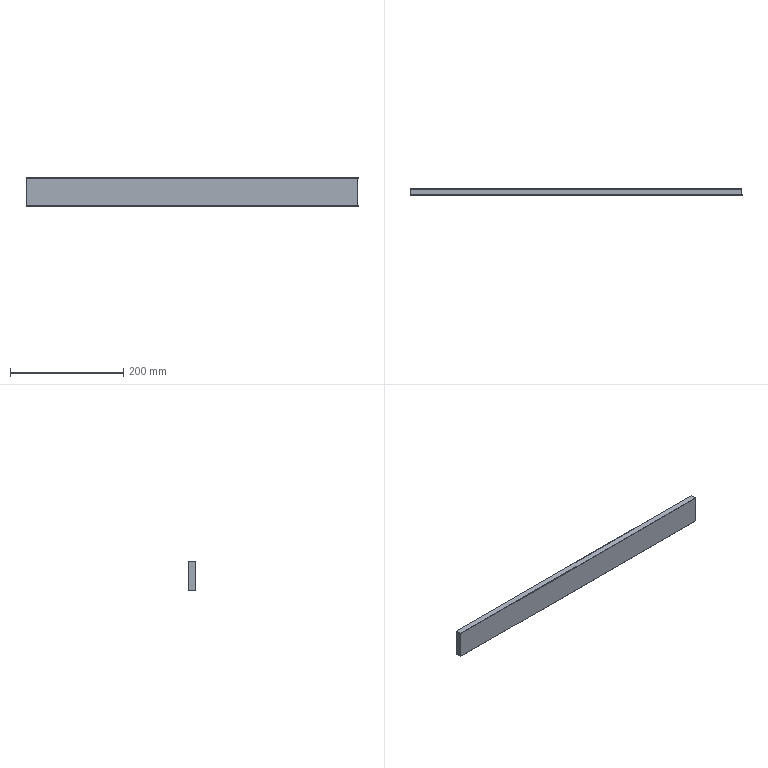Part | STEP file | DEWALT-DWE7492-B22 | 1 solid | 10 faces | box 586.2 x 11 x 50 mm | volume 322284 mm3 | plane 6 | cylinder 4 | commonest cylinder face diameters 1 x4
STEP:
#1=CARTESIAN_POINT('',(0.,0.,0.));
#2=DIRECTION('',(0.,0.,1.));
#3=DIRECTION('',(1.,0.,0.));
#4=AXIS2_PLACEMENT_3D('',#1,#2,#3);
#5=CARTESIAN_POINT('',(-302.1,210.8,45.5));
#6=VERTEX_POINT('',#5);
#7=CARTESIAN_POINT('',(-302.1,211.3,45.));
#8=VERTEX_POINT('',#7);
#9=CARTESIAN_POINT('',(-302.1,211.3,45.5));
#10=DIRECTION('',(1.,0.,0.));
#11=DIRECTION('',(0.,-1.,0.));
#12=AXIS2_PLACEMENT_3D('',#9,#10,#11);
#13=CIRCLE('',#12,0.5);
#14=CARTESIAN_POINT('',(-302.1,211.3,45.5));
#15=DIRECTION('',(1.,0.,0.));
#16=DIRECTION('',(0.,0.,-1.));
#17=AXIS2_PLACEMENT_3D('',#14,#15,#16);
#18=CYLINDRICAL_SURFACE('',#17,0.5);
#19=CARTESIAN_POINT('',(4.712,0.));
#20=DIRECTION('',(1.,0.));
#21=VECTOR('',#20,1.);
#22=LINE('',#19,#21);
#23=(GEOMETRIC_REPRESENTATION_CONTEXT(2)PARAMETRIC_REPRESENTATION_CONTEXT()REPRESENTATION_CONTEXT('',''));
#24=DEFINITIONAL_REPRESENTATION('',(#22),#23);
#25=PCURVE('',#18,#24);
#26=CARTESIAN_POINT('',(-302.1,210.79,44.99));
#27=DIRECTION('',(-1.,0.,0.));
#28=DIRECTION('',(0.,0.,1.));
#29=AXIS2_PLACEMENT_3D('',#26,#27,#28);
#30=PLANE('',#29);
#31=CARTESIAN_POINT('',(0.51,0.01));
#32=CARTESIAN_POINT('',(-0.356,0.01));
#33=CARTESIAN_POINT('',(0.07699,0.76));
#34=CARTESIAN_POINT('',(0.51,1.51));
#35=CARTESIAN_POINT('',(0.943,0.76));
#36=CARTESIAN_POINT('',(1.376,0.01));
#37=CARTESIAN_POINT('',(0.51,0.01));
#38=(BOUNDED_CURVE()B_SPLINE_CURVE(2,(#31,#32,#33,#34,#35,#36,#37),.UNSPECIFIED.,.T.,.F.)B_SPLINE_CURVE_WITH_KNOTS((1,2,2,2,2,1),(-2.094,0.,2.094,4.189,6.283,8.378),.UNSPECIFIED.)CURVE()GEOMETRIC_REPRESENTATION_ITEM()RATIONAL_B_SPLINE_CURVE((1.,0.5,1.,0.5,1.,0.5,1.))REPRESENTATION_ITEM(''));
#39=(GEOMETRIC_REPRESENTATION_CONTEXT(2)PARAMETRIC_REPRESENTATION_CONTEXT()REPRESENTATION_CONTEXT('',''));
#40=DEFINITIONAL_REPRESENTATION('',(#38),#39);
#41=PCURVE('',#30,#40);
#42=SURFACE_CURVE('',#13,(#25,#41),.PCURVE_S1.);
#43=EDGE_CURVE('',#6,#8,#42,.T.);
#44=ORIENTED_EDGE('',*,*,#43,.T.);
#45=CARTESIAN_POINT('',(284.1,211.3,45.));
#46=VERTEX_POINT('',#45);
#47=CARTESIAN_POINT('',(-9.,211.3,45.));
#48=DIRECTION('',(1.,0.,0.));
#49=VECTOR('',#48,1.);
#50=LINE('',#47,#49);
#51=CARTESIAN_POINT('',(6.283,293.1));
#52=DIRECTION('',(0.,1.));
#53=VECTOR('',#52,1.);
#54=LINE('',#51,#53);
#55=(GEOMETRIC_REPRESENTATION_CONTEXT(2)PARAMETRIC_REPRESENTATION_CONTEXT()REPRESENTATION_CONTEXT('',''));
#56=DEFINITIONAL_REPRESENTATION('',(#54),#55);
#57=PCURVE('',#18,#56);
#58=CARTESIAN_POINT('',(284.11,221.31,45.));
#59=DIRECTION('',(0.,0.,-1.));
#60=DIRECTION('',(0.,-1.,0.));
#61=AXIS2_PLACEMENT_3D('',#58,#59,#60);
#62=PLANE('',#61);
#63=CARTESIAN_POINT('',(10.01,293.11));
#64=DIRECTION('',(0.,-1.));
#65=VECTOR('',#64,1.);
#66=LINE('',#63,#65);
#67=(GEOMETRIC_REPRESENTATION_CONTEXT(2)PARAMETRIC_REPRESENTATION_CONTEXT()REPRESENTATION_CONTEXT('',''));
#68=DEFINITIONAL_REPRESENTATION('',(#66),#67);
#69=PCURVE('',#62,#68);
#70=SURFACE_CURVE('',#50,(#57,#69),.PCURVE_S1.);
#71=EDGE_CURVE('',#8,#46,#70,.T.);
#72=ORIENTED_EDGE('',*,*,#71,.T.);
#73=CARTESIAN_POINT('',(284.1,210.8,45.5));
#74=VERTEX_POINT('',#73);
#75=CARTESIAN_POINT('',(284.1,211.3,45.5));
#76=DIRECTION('',(-1.,0.,0.));
#77=DIRECTION('',(0.,0.,-1.));
#78=AXIS2_PLACEMENT_3D('',#75,#76,#77);
#79=CIRCLE('',#78,0.5);
#80=CARTESIAN_POINT('',(6.283,586.2));
#81=DIRECTION('',(-1.,0.));
#82=VECTOR('',#81,1.);
#83=LINE('',#80,#82);
#84=(GEOMETRIC_REPRESENTATION_CONTEXT(2)PARAMETRIC_REPRESENTATION_CONTEXT()REPRESENTATION_CONTEXT('',''));
#85=DEFINITIONAL_REPRESENTATION('',(#83),#84);
#86=PCURVE('',#18,#85);
#87=CARTESIAN_POINT('',(284.1,210.79,44.99));
#88=DIRECTION('',(1.,0.,0.));
#89=DIRECTION('',(0.,1.,0.));
#90=AXIS2_PLACEMENT_3D('',#87,#88,#89);
#91=PLANE('',#90);
#92=CARTESIAN_POINT('',(0.51,0.01));
#93=CARTESIAN_POINT('',(-0.356,0.01));
#94=CARTESIAN_POINT('',(0.07699,0.76));
#95=CARTESIAN_POINT('',(0.51,1.51));
#96=CARTESIAN_POINT('',(0.943,0.76));
#97=CARTESIAN_POINT('',(1.376,0.01));
#98=CARTESIAN_POINT('',(0.51,0.01));
#99=(BOUNDED_CURVE()B_SPLINE_CURVE(2,(#92,#93,#94,#95,#96,#97,#98),.UNSPECIFIED.,.T.,.F.)B_SPLINE_CURVE_WITH_KNOTS((1,2,2,2,2,1),(-2.094,0.,2.094,4.189,6.283,8.378),.UNSPECIFIED.)CURVE()GEOMETRIC_REPRESENTATION_ITEM()RATIONAL_B_SPLINE_CURVE((1.,0.5,1.,0.5,1.,0.5,1.))REPRESENTATION_ITEM(''));
#100=(GEOMETRIC_REPRESENTATION_CONTEXT(2)PARAMETRIC_REPRESENTATION_CONTEXT()REPRESENTATION_CONTEXT('',''));
#101=DEFINITIONAL_REPRESENTATION('',(#99),#100);
#102=PCURVE('',#91,#101);
#103=SURFACE_CURVE('',#79,(#86,#102),.PCURVE_S1.);
#104=EDGE_CURVE('',#46,#74,#103,.T.);
#105=ORIENTED_EDGE('',*,*,#104,.T.);
#106=CARTESIAN_POINT('',(-9.,210.8,45.5));
#107=DIRECTION('',(-1.,0.,0.));
#108=VECTOR('',#107,1.);
#109=LINE('',#106,#108);
#110=CARTESIAN_POINT('',(4.712,293.1));
#111=DIRECTION('',(0.,-1.));
#112=VECTOR('',#111,1.);
#113=LINE('',#110,#112);
#114=(GEOMETRIC_REPRESENTATION_CONTEXT(2)PARAMETRIC_REPRESENTATION_CONTEXT()REPRESENTATION_CONTEXT('',''));
#115=DEFINITIONAL_REPRESENTATION('',(#113),#114);
#116=PCURVE('',#18,#115);
#117=CARTESIAN_POINT('',(284.11,210.8,45.49));
#118=DIRECTION('',(0.,-1.,0.));
#119=DIRECTION('',(0.,0.,1.));
#120=AXIS2_PLACEMENT_3D('',#117,#118,#119);
#121=PLANE('',#120);
#122=CARTESIAN_POINT('',(0.01,293.11));
#123=DIRECTION('',(0.,1.));
#124=VECTOR('',#123,1.);
#125=LINE('',#122,#124);
#126=(GEOMETRIC_REPRESENTATION_CONTEXT(2)PARAMETRIC_REPRESENTATION_CONTEXT()REPRESENTATION_CONTEXT('',''));
#127=DEFINITIONAL_REPRESENTATION('',(#125),#126);
#128=PCURVE('',#121,#127);
#129=SURFACE_CURVE('',#109,(#116,#128),.PCURVE_S1.);
#130=EDGE_CURVE('',#74,#6,#129,.T.);
#131=ORIENTED_EDGE('',*,*,#130,.T.);
#132=EDGE_LOOP('',(#44,#72,#105,#131));
#133=FACE_BOUND('',#132,.T.);
#134=ADVANCED_FACE('',(#133),#18,.T.);
#135=ORIENTED_EDGE('',*,*,#130,.F.);
#136=CARTESIAN_POINT('',(284.1,210.8,94.5));
#137=VERTEX_POINT('',#136);
#138=CARTESIAN_POINT('',(284.1,210.8,70.));
#139=DIRECTION('',(0.,0.,-1.));
#140=VECTOR('',#139,1.);
#141=LINE('',#138,#140);
#142=CARTESIAN_POINT('',(24.51,0.01));
#143=DIRECTION('',(-1.,0.));
#144=VECTOR('',#143,1.);
#145=LINE('',#142,#144);
#146=(GEOMETRIC_REPRESENTATION_CONTEXT(2)PARAMETRIC_REPRESENTATION_CONTEXT()REPRESENTATION_CONTEXT('',''));
#147=DEFINITIONAL_REPRESENTATION('',(#145),#146);
#148=PCURVE('',#121,#147);
#149=CARTESIAN_POINT('',(0.01,25.01));
#150=DIRECTION('',(0.,-1.));
#151=VECTOR('',#150,1.);
#152=LINE('',#149,#151);
#153=(GEOMETRIC_REPRESENTATION_CONTEXT(2)PARAMETRIC_REPRESENTATION_CONTEXT()REPRESENTATION_CONTEXT('',''));
#154=DEFINITIONAL_REPRESENTATION('',(#152),#153);
#155=PCURVE('',#91,#154);
#156=SURFACE_CURVE('',#141,(#148,#155),.PCURVE_S1.);
#157=EDGE_CURVE('',#137,#74,#156,.T.);
#158=ORIENTED_EDGE('',*,*,#157,.F.);
#159=CARTESIAN_POINT('',(-302.1,210.8,94.5));
#160=VERTEX_POINT('',#159);
#161=CARTESIAN_POINT('',(-9.,210.8,94.5));
#162=DIRECTION('',(1.,0.,0.));
#163=VECTOR('',#162,1.);
#164=LINE('',#161,#163);
#165=CARTESIAN_POINT('',(49.01,293.11));
#166=DIRECTION('',(0.,-1.));
#167=VECTOR('',#166,1.);
#168=LINE('',#165,#167);
#169=(GEOMETRIC_REPRESENTATION_CONTEXT(2)PARAMETRIC_REPRESENTATION_CONTEXT()REPRESENTATION_CONTEXT('',''));
#170=DEFINITIONAL_REPRESENTATION('',(#168),#169);
#171=PCURVE('',#121,#170);
#172=CARTESIAN_POINT('',(-302.1,211.3,94.5));
#173=DIRECTION('',(1.,0.,0.));
#174=DIRECTION('',(0.,0.,-1.));
#175=AXIS2_PLACEMENT_3D('',#172,#173,#174);
#176=CYLINDRICAL_SURFACE('',#175,0.5);
#177=CARTESIAN_POINT('',(4.712,293.1));
#178=DIRECTION('',(0.,1.));
#179=VECTOR('',#178,1.);
#180=LINE('',#177,#179);
#181=(GEOMETRIC_REPRESENTATION_CONTEXT(2)PARAMETRIC_REPRESENTATION_CONTEXT()REPRESENTATION_CONTEXT('',''));
#182=DEFINITIONAL_REPRESENTATION('',(#180),#181);
#183=PCURVE('',#176,#182);
#184=SURFACE_CURVE('',#164,(#171,#183),.PCURVE_S1.);
#185=EDGE_CURVE('',#160,#137,#184,.T.);
#186=ORIENTED_EDGE('',*,*,#185,.F.);
#187=CARTESIAN_POINT('',(-302.1,210.8,70.));
#188=DIRECTION('',(0.,0.,1.));
#189=VECTOR('',#188,1.);
#190=LINE('',#187,#189);
#191=CARTESIAN_POINT('',(24.51,586.21));
#192=DIRECTION('',(1.,0.));
#193=VECTOR('',#192,1.);
#194=LINE('',#191,#193);
#195=(GEOMETRIC_REPRESENTATION_CONTEXT(2)PARAMETRIC_REPRESENTATION_CONTEXT()REPRESENTATION_CONTEXT('',''));
#196=DEFINITIONAL_REPRESENTATION('',(#194),#195);
#197=PCURVE('',#121,#196);
#198=CARTESIAN_POINT('',(25.01,0.01));
#199=DIRECTION('',(1.,0.));
#200=VECTOR('',#199,1.);
#201=LINE('',#198,#200);
#202=(GEOMETRIC_REPRESENTATION_CONTEXT(2)PARAMETRIC_REPRESENTATION_CONTEXT()REPRESENTATION_CONTEXT('',''));
#203=DEFINITIONAL_REPRESENTATION('',(#201),#202);
#204=PCURVE('',#30,#203);
#205=SURFACE_CURVE('',#190,(#197,#204),.PCURVE_S1.);
#206=EDGE_CURVE('',#6,#160,#205,.T.);
#207=ORIENTED_EDGE('',*,*,#206,.F.);
#208=EDGE_LOOP('',(#135,#158,#186,#207));
#209=FACE_BOUND('',#208,.T.);
#210=ADVANCED_FACE('',(#209),#121,.T.);
#211=ORIENTED_EDGE('',*,*,#104,.F.);
#212=CARTESIAN_POINT('',(284.1,221.3,45.));
#213=VERTEX_POINT('',#212);
#214=CARTESIAN_POINT('',(284.1,216.3,45.));
#215=DIRECTION('',(0.,1.,0.));
#216=VECTOR('',#215,1.);
#217=LINE('',#214,#216);
#218=CARTESIAN_POINT('',(5.51,0.01));
#219=DIRECTION('',(1.,0.));
#220=VECTOR('',#219,1.);
#221=LINE('',#218,#220);
#222=(GEOMETRIC_REPRESENTATION_CONTEXT(2)PARAMETRIC_REPRESENTATION_CONTEXT()REPRESENTATION_CONTEXT('',''));
#223=DEFINITIONAL_REPRESENTATION('',(#221),#222);
#224=PCURVE('',#91,#223);
#225=CARTESIAN_POINT('',(5.01,0.01));
#226=DIRECTION('',(-1.,0.));
#227=VECTOR('',#226,1.);
#228=LINE('',#225,#227);
#229=(GEOMETRIC_REPRESENTATION_CONTEXT(2)PARAMETRIC_REPRESENTATION_CONTEXT()REPRESENTATION_CONTEXT('',''));
#230=DEFINITIONAL_REPRESENTATION('',(#228),#229);
#231=PCURVE('',#62,#230);
#232=SURFACE_CURVE('',#217,(#224,#231),.PCURVE_S1.);
#233=EDGE_CURVE('',#46,#213,#232,.T.);
#234=ORIENTED_EDGE('',*,*,#233,.T.);
#235=CARTESIAN_POINT('',(284.1,221.8,45.5));
#236=VERTEX_POINT('',#235);
#237=CARTESIAN_POINT('',(284.1,221.3,45.5));
#238=DIRECTION('',(-1.,0.,0.));
#239=DIRECTION('',(0.,1.,0.));
#240=AXIS2_PLACEMENT_3D('',#237,#238,#239);
#241=CIRCLE('',#240,0.5);
#242=CARTESIAN_POINT('',(11.01,0.51));
#243=CARTESIAN_POINT('',(11.01,-0.356));
#244=CARTESIAN_POINT('',(10.26,0.07699));
#245=CARTESIAN_POINT('',(9.51,0.51));
#246=CARTESIAN_POINT('',(10.26,0.943));
#247=CARTESIAN_POINT('',(11.01,1.376));
#248=CARTESIAN_POINT('',(11.01,0.51));
#249=(BOUNDED_CURVE()B_SPLINE_CURVE(2,(#242,#243,#244,#245,#246,#247,#248),.UNSPECIFIED.,.T.,.F.)B_SPLINE_CURVE_WITH_KNOTS((1,2,2,2,2,1),(-2.094,0.,2.094,4.189,6.283,8.378),.UNSPECIFIED.)CURVE()GEOMETRIC_REPRESENTATION_ITEM()RATIONAL_B_SPLINE_CURVE((1.,0.5,1.,0.5,1.,0.5,1.))REPRESENTATION_ITEM(''));
#250=(GEOMETRIC_REPRESENTATION_CONTEXT(2)PARAMETRIC_REPRESENTATION_CONTEXT()REPRESENTATION_CONTEXT('',''));
#251=DEFINITIONAL_REPRESENTATION('',(#249),#250);
#252=PCURVE('',#91,#251);
#253=CARTESIAN_POINT('',(-302.1,221.3,45.5));
#254=DIRECTION('',(1.,0.,0.));
#255=DIRECTION('',(0.,1.,0.));
#256=AXIS2_PLACEMENT_3D('',#253,#254,#255);
#257=CYLINDRICAL_SURFACE('',#256,0.5);
#258=CARTESIAN_POINT('',(6.283,586.2));
#259=DIRECTION('',(-1.,0.));
#260=VECTOR('',#259,1.);
#261=LINE('',#258,#260);
#262=(GEOMETRIC_REPRESENTATION_CONTEXT(2)PARAMETRIC_REPRESENTATION_CONTEXT()REPRESENTATION_CONTEXT('',''));
#263=DEFINITIONAL_REPRESENTATION('',(#261),#262);
#264=PCURVE('',#257,#263);
#265=SURFACE_CURVE('',#241,(#252,#264),.PCURVE_S1.);
#266=EDGE_CURVE('',#236,#213,#265,.T.);
#267=ORIENTED_EDGE('',*,*,#266,.F.);
#268=CARTESIAN_POINT('',(284.1,221.8,94.5));
#269=VERTEX_POINT('',#268);
#270=CARTESIAN_POINT('',(284.1,221.8,70.));
#271=DIRECTION('',(0.,0.,1.));
#272=VECTOR('',#271,1.);
#273=LINE('',#270,#272);
#274=CARTESIAN_POINT('',(11.01,25.01));
#275=DIRECTION('',(0.,1.));
#276=VECTOR('',#275,1.);
#277=LINE('',#274,#276);
#278=(GEOMETRIC_REPRESENTATION_CONTEXT(2)PARAMETRIC_REPRESENTATION_CONTEXT()REPRESENTATION_CONTEXT('',''));
#279=DEFINITIONAL_REPRESENTATION('',(#277),#278);
#280=PCURVE('',#91,#279);
#281=CARTESIAN_POINT('',(284.11,221.8,94.51));
#282=DIRECTION('',(0.,1.,0.));
#283=DIRECTION('',(0.,0.,-1.));
#284=AXIS2_PLACEMENT_3D('',#281,#282,#283);
#285=PLANE('',#284);
#286=CARTESIAN_POINT('',(24.51,0.01));
#287=DIRECTION('',(-1.,0.));
#288=VECTOR('',#287,1.);
#289=LINE('',#286,#288);
#290=(GEOMETRIC_REPRESENTATION_CONTEXT(2)PARAMETRIC_REPRESENTATION_CONTEXT()REPRESENTATION_CONTEXT('',''));
#291=DEFINITIONAL_REPRESENTATION('',(#289),#290);
#292=PCURVE('',#285,#291);
#293=SURFACE_CURVE('',#273,(#280,#292),.PCURVE_S1.);
#294=EDGE_CURVE('',#236,#269,#293,.T.);
#295=ORIENTED_EDGE('',*,*,#294,.T.);
#296=CARTESIAN_POINT('',(284.1,221.3,95.));
#297=VERTEX_POINT('',#296);
#298=CARTESIAN_POINT('',(284.1,221.3,94.5));
#299=DIRECTION('',(-1.,0.,0.));
#300=DIRECTION('',(0.,0.,1.));
#301=AXIS2_PLACEMENT_3D('',#298,#299,#300);
#302=CIRCLE('',#301,0.5);
#303=CARTESIAN_POINT('',(10.51,50.01));
#304=CARTESIAN_POINT('',(11.376,50.01));
#305=CARTESIAN_POINT('',(10.943,49.26));
#306=CARTESIAN_POINT('',(10.51,48.51));
#307=CARTESIAN_POINT('',(10.077,49.26));
#308=CARTESIAN_POINT('',(9.644,50.01));
#309=CARTESIAN_POINT('',(10.51,50.01));
#310=(BOUNDED_CURVE()B_SPLINE_CURVE(2,(#303,#304,#305,#306,#307,#308,#309),.UNSPECIFIED.,.T.,.F.)B_SPLINE_CURVE_WITH_KNOTS((1,2,2,2,2,1),(-2.094,0.,2.094,4.189,6.283,8.378),.UNSPECIFIED.)CURVE()GEOMETRIC_REPRESENTATION_ITEM()RATIONAL_B_SPLINE_CURVE((1.,0.5,1.,0.5,1.,0.5,1.))REPRESENTATION_ITEM(''));
#311=(GEOMETRIC_REPRESENTATION_CONTEXT(2)PARAMETRIC_REPRESENTATION_CONTEXT()REPRESENTATION_CONTEXT('',''));
#312=DEFINITIONAL_REPRESENTATION('',(#310),#311);
#313=PCURVE('',#91,#312);
#314=CARTESIAN_POINT('',(-302.1,221.3,94.5));
#315=DIRECTION('',(1.,0.,0.));
#316=DIRECTION('',(0.,1.,0.));
#317=AXIS2_PLACEMENT_3D('',#314,#315,#316);
#318=CYLINDRICAL_SURFACE('',#317,0.5);
#319=CARTESIAN_POINT('',(1.571,586.2));
#320=DIRECTION('',(-1.,0.));
#321=VECTOR('',#320,1.);
#322=LINE('',#319,#321);
#323=(GEOMETRIC_REPRESENTATION_CONTEXT(2)PARAMETRIC_REPRESENTATION_CONTEXT()REPRESENTATION_CONTEXT('',''));
#324=DEFINITIONAL_REPRESENTATION('',(#322),#323);
#325=PCURVE('',#318,#324);
#326=SURFACE_CURVE('',#302,(#313,#325),.PCURVE_S1.);
#327=EDGE_CURVE('',#297,#269,#326,.T.);
#328=ORIENTED_EDGE('',*,*,#327,.F.);
#329=CARTESIAN_POINT('',(284.1,211.3,95.));
#330=VERTEX_POINT('',#329);
#331=CARTESIAN_POINT('',(284.1,216.3,95.));
#332=DIRECTION('',(0.,-1.,0.));
#333=VECTOR('',#332,1.);
#334=LINE('',#331,#333);
#335=CARTESIAN_POINT('',(5.51,50.01));
#336=DIRECTION('',(-1.,0.));
#337=VECTOR('',#336,1.);
#338=LINE('',#335,#337);
#339=(GEOMETRIC_REPRESENTATION_CONTEXT(2)PARAMETRIC_REPRESENTATION_CONTEXT()REPRESENTATION_CONTEXT('',''));
#340=DEFINITIONAL_REPRESENTATION('',(#338),#339);
#341=PCURVE('',#91,#340);
#342=CARTESIAN_POINT('',(284.11,211.29,95.));
#343=DIRECTION('',(0.,0.,1.));
#344=DIRECTION('',(0.,1.,0.));
#345=AXIS2_PLACEMENT_3D('',#342,#343,#344);
#346=PLANE('',#345);
#347=CARTESIAN_POINT('',(5.01,0.01));
#348=DIRECTION('',(-1.,0.));
#349=VECTOR('',#348,1.);
#350=LINE('',#347,#349);
#351=(GEOMETRIC_REPRESENTATION_CONTEXT(2)PARAMETRIC_REPRESENTATION_CONTEXT()REPRESENTATION_CONTEXT('',''));
#352=DEFINITIONAL_REPRESENTATION('',(#350),#351);
#353=PCURVE('',#346,#352);
#354=SURFACE_CURVE('',#334,(#341,#353),.PCURVE_S1.);
#355=EDGE_CURVE('',#297,#330,#354,.T.);
#356=ORIENTED_EDGE('',*,*,#355,.T.);
#357=CARTESIAN_POINT('',(284.1,211.3,94.5));
#358=DIRECTION('',(-1.,0.,0.));
#359=DIRECTION('',(0.,-1.,0.));
#360=AXIS2_PLACEMENT_3D('',#357,#358,#359);
#361=CIRCLE('',#360,0.5);
#362=CARTESIAN_POINT('',(0.01,49.51));
#363=CARTESIAN_POINT('',(0.01,50.376));
#364=CARTESIAN_POINT('',(0.76,49.943));
#365=CARTESIAN_POINT('',(1.51,49.51));
#366=CARTESIAN_POINT('',(0.76,49.077));
#367=CARTESIAN_POINT('',(0.01,48.644));
#368=CARTESIAN_POINT('',(0.01,49.51));
#369=(BOUNDED_CURVE()B_SPLINE_CURVE(2,(#362,#363,#364,#365,#366,#367,#368),.UNSPECIFIED.,.T.,.F.)B_SPLINE_CURVE_WITH_KNOTS((1,2,2,2,2,1),(-2.094,0.,2.094,4.189,6.283,8.378),.UNSPECIFIED.)CURVE()GEOMETRIC_REPRESENTATION_ITEM()RATIONAL_B_SPLINE_CURVE((1.,0.5,1.,0.5,1.,0.5,1.))REPRESENTATION_ITEM(''));
#370=(GEOMETRIC_REPRESENTATION_CONTEXT(2)PARAMETRIC_REPRESENTATION_CONTEXT()REPRESENTATION_CONTEXT('',''));
#371=DEFINITIONAL_REPRESENTATION('',(#369),#370);
#372=PCURVE('',#91,#371);
#373=CARTESIAN_POINT('',(4.712,586.2));
#374=CARTESIAN_POINT('',(3.142,586.2));
#375=B_SPLINE_CURVE_WITH_KNOTS('',1,(#373,#374),.UNSPECIFIED.,.F.,.F.,(2,2),(0.,1.571),.PIECEWISE_BEZIER_KNOTS.);
#376=(GEOMETRIC_REPRESENTATION_CONTEXT(2)PARAMETRIC_REPRESENTATION_CONTEXT()REPRESENTATION_CONTEXT('',''));
#377=DEFINITIONAL_REPRESENTATION('',(#375),#376);
#378=PCURVE('',#176,#377);
#379=SURFACE_CURVE('',#361,(#372,#378),.PCURVE_S1.);
#380=EDGE_CURVE('',#137,#330,#379,.T.);
#381=ORIENTED_EDGE('',*,*,#380,.F.);
#382=ORIENTED_EDGE('',*,*,#157,.T.);
#383=EDGE_LOOP('',(#211,#234,#267,#295,#328,#356,#381,#382));
#384=FACE_BOUND('',#383,.T.);
#385=ADVANCED_FACE('',(#384),#91,.T.);
#386=CARTESIAN_POINT('',(-302.1,221.3,45.));
#387=VERTEX_POINT('',#386);
#388=CARTESIAN_POINT('',(-302.1,221.8,45.5));
#389=VERTEX_POINT('',#388);
#390=CARTESIAN_POINT('',(-302.1,221.3,45.5));
#391=DIRECTION('',(1.,0.,0.));
#392=DIRECTION('',(0.,0.,-1.));
#393=AXIS2_PLACEMENT_3D('',#390,#391,#392);
#394=CIRCLE('',#393,0.5);
#395=CARTESIAN_POINT('',(4.712,0.));
#396=DIRECTION('',(1.,0.));
#397=VECTOR('',#396,1.);
#398=LINE('',#395,#397);
#399=(GEOMETRIC_REPRESENTATION_CONTEXT(2)PARAMETRIC_REPRESENTATION_CONTEXT()REPRESENTATION_CONTEXT('',''));
#400=DEFINITIONAL_REPRESENTATION('',(#398),#399);
#401=PCURVE('',#257,#400);
#402=CARTESIAN_POINT('',(0.01,10.51));
#403=CARTESIAN_POINT('',(0.01,11.376));
#404=CARTESIAN_POINT('',(0.76,10.943));
#405=CARTESIAN_POINT('',(1.51,10.51));
#406=CARTESIAN_POINT('',(0.76,10.077));
#407=CARTESIAN_POINT('',(0.01,9.644));
#408=CARTESIAN_POINT('',(0.01,10.51));
#409=(BOUNDED_CURVE()B_SPLINE_CURVE(2,(#402,#403,#404,#405,#406,#407,#408),.UNSPECIFIED.,.T.,.F.)B_SPLINE_CURVE_WITH_KNOTS((1,2,2,2,2,1),(-2.094,0.,2.094,4.189,6.283,8.378),.UNSPECIFIED.)CURVE()GEOMETRIC_REPRESENTATION_ITEM()RATIONAL_B_SPLINE_CURVE((1.,0.5,1.,0.5,1.,0.5,1.))REPRESENTATION_ITEM(''));
#410=(GEOMETRIC_REPRESENTATION_CONTEXT(2)PARAMETRIC_REPRESENTATION_CONTEXT()REPRESENTATION_CONTEXT('',''));
#411=DEFINITIONAL_REPRESENTATION('',(#409),#410);
#412=PCURVE('',#30,#411);
#413=SURFACE_CURVE('',#394,(#401,#412),.PCURVE_S1.);
#414=EDGE_CURVE('',#387,#389,#413,.T.);
#415=ORIENTED_EDGE('',*,*,#414,.T.);
#416=CARTESIAN_POINT('',(-9.,221.8,45.5));
#417=DIRECTION('',(1.,0.,0.));
#418=VECTOR('',#417,1.);
#419=LINE('',#416,#418);
#420=CARTESIAN_POINT('',(6.283,293.1));
#421=DIRECTION('',(0.,1.));
#422=VECTOR('',#421,1.);
#423=LINE('',#420,#422);
#424=(GEOMETRIC_REPRESENTATION_CONTEXT(2)PARAMETRIC_REPRESENTATION_CONTEXT()REPRESENTATION_CONTEXT('',''));
#425=DEFINITIONAL_REPRESENTATION('',(#423),#424);
#426=PCURVE('',#257,#425);
#427=CARTESIAN_POINT('',(49.01,293.11));
#428=DIRECTION('',(0.,-1.));
#429=VECTOR('',#428,1.);
#430=LINE('',#427,#429);
#431=(GEOMETRIC_REPRESENTATION_CONTEXT(2)PARAMETRIC_REPRESENTATION_CONTEXT()REPRESENTATION_CONTEXT('',''));
#432=DEFINITIONAL_REPRESENTATION('',(#430),#431);
#433=PCURVE('',#285,#432);
#434=SURFACE_CURVE('',#419,(#426,#433),.PCURVE_S1.);
#435=EDGE_CURVE('',#389,#236,#434,.T.);
#436=ORIENTED_EDGE('',*,*,#435,.T.);
#437=ORIENTED_EDGE('',*,*,#266,.T.);
#438=CARTESIAN_POINT('',(-9.,221.3,45.));
#439=DIRECTION('',(-1.,0.,0.));
#440=VECTOR('',#439,1.);
#441=LINE('',#438,#440);
#442=CARTESIAN_POINT('',(4.712,293.1));
#443=DIRECTION('',(0.,-1.));
#444=VECTOR('',#443,1.);
#445=LINE('',#442,#444);
#446=(GEOMETRIC_REPRESENTATION_CONTEXT(2)PARAMETRIC_REPRESENTATION_CONTEXT()REPRESENTATION_CONTEXT('',''));
#447=DEFINITIONAL_REPRESENTATION('',(#445),#446);
#448=PCURVE('',#257,#447);
#449=CARTESIAN_POINT('',(0.01,293.11));
#450=DIRECTION('',(0.,1.));
#451=VECTOR('',#450,1.);
#452=LINE('',#449,#451);
#453=(GEOMETRIC_REPRESENTATION_CONTEXT(2)PARAMETRIC_REPRESENTATION_CONTEXT()REPRESENTATION_CONTEXT('',''));
#454=DEFINITIONAL_REPRESENTATION('',(#452),#453);
#455=PCURVE('',#62,#454);
#456=SURFACE_CURVE('',#441,(#448,#455),.PCURVE_S1.);
#457=EDGE_CURVE('',#213,#387,#456,.T.);
#458=ORIENTED_EDGE('',*,*,#457,.T.);
#459=EDGE_LOOP('',(#415,#436,#437,#458));
#460=FACE_BOUND('',#459,.T.);
#461=ADVANCED_FACE('',(#460),#257,.T.);
#462=ORIENTED_EDGE('',*,*,#435,.F.);
#463=CARTESIAN_POINT('',(-302.1,221.8,94.5));
#464=VERTEX_POINT('',#463);
#465=CARTESIAN_POINT('',(-302.1,221.8,70.));
#466=DIRECTION('',(0.,0.,-1.));
#467=VECTOR('',#466,1.);
#468=LINE('',#465,#467);
#469=CARTESIAN_POINT('',(24.51,586.21));
#470=DIRECTION('',(1.,0.));
#471=VECTOR('',#470,1.);
#472=LINE('',#469,#471);
#473=(GEOMETRIC_REPRESENTATION_CONTEXT(2)PARAMETRIC_REPRESENTATION_CONTEXT()REPRESENTATION_CONTEXT('',''));
#474=DEFINITIONAL_REPRESENTATION('',(#472),#473);
#475=PCURVE('',#285,#474);
#476=CARTESIAN_POINT('',(25.01,11.01));
#477=DIRECTION('',(-1.,0.));
#478=VECTOR('',#477,1.);
#479=LINE('',#476,#478);
#480=(GEOMETRIC_REPRESENTATION_CONTEXT(2)PARAMETRIC_REPRESENTATION_CONTEXT()REPRESENTATION_CONTEXT('',''));
#481=DEFINITIONAL_REPRESENTATION('',(#479),#480);
#482=PCURVE('',#30,#481);
#483=SURFACE_CURVE('',#468,(#475,#482),.PCURVE_S1.);
#484=EDGE_CURVE('',#464,#389,#483,.T.);
#485=ORIENTED_EDGE('',*,*,#484,.F.);
#486=CARTESIAN_POINT('',(-9.,221.8,94.5));
#487=DIRECTION('',(-1.,0.,0.));
#488=VECTOR('',#487,1.);
#489=LINE('',#486,#488);
#490=CARTESIAN_POINT('',(0.01,293.11));
#491=DIRECTION('',(0.,1.));
#492=VECTOR('',#491,1.);
#493=LINE('',#490,#492);
#494=(GEOMETRIC_REPRESENTATION_CONTEXT(2)PARAMETRIC_REPRESENTATION_CONTEXT()REPRESENTATION_CONTEXT('',''));
#495=DEFINITIONAL_REPRESENTATION('',(#493),#494);
#496=PCURVE('',#285,#495);
#497=CARTESIAN_POINT('',(0.,293.1));
#498=DIRECTION('',(0.,-1.));
#499=VECTOR('',#498,1.);
#500=LINE('',#497,#499);
#501=(GEOMETRIC_REPRESENTATION_CONTEXT(2)PARAMETRIC_REPRESENTATION_CONTEXT()REPRESENTATION_CONTEXT('',''));
#502=DEFINITIONAL_REPRESENTATION('',(#500),#501);
#503=PCURVE('',#318,#502);
#504=SURFACE_CURVE('',#489,(#496,#503),.PCURVE_S1.);
#505=EDGE_CURVE('',#269,#464,#504,.T.);
#506=ORIENTED_EDGE('',*,*,#505,.F.);
#507=ORIENTED_EDGE('',*,*,#294,.F.);
#508=EDGE_LOOP('',(#462,#485,#506,#507));
#509=FACE_BOUND('',#508,.T.);
#510=ADVANCED_FACE('',(#509),#285,.T.);
#511=CARTESIAN_POINT('',(-302.1,221.3,95.));
#512=VERTEX_POINT('',#511);
#513=CARTESIAN_POINT('',(-302.1,221.3,94.5));
#514=DIRECTION('',(1.,0.,0.));
#515=DIRECTION('',(0.,1.,0.));
#516=AXIS2_PLACEMENT_3D('',#513,#514,#515);
#517=CIRCLE('',#516,0.5);
#518=CARTESIAN_POINT('',(0.,0.));
#519=DIRECTION('',(1.,0.));
#520=VECTOR('',#519,1.);
#521=LINE('',#518,#520);
#522=(GEOMETRIC_REPRESENTATION_CONTEXT(2)PARAMETRIC_REPRESENTATION_CONTEXT()REPRESENTATION_CONTEXT('',''));
#523=DEFINITIONAL_REPRESENTATION('',(#521),#522);
#524=PCURVE('',#318,#523);
#525=CARTESIAN_POINT('',(49.51,11.01));
#526=CARTESIAN_POINT('',(50.376,11.01));
#527=CARTESIAN_POINT('',(49.943,10.26));
#528=CARTESIAN_POINT('',(49.51,9.51));
#529=CARTESIAN_POINT('',(49.077,10.26));
#530=CARTESIAN_POINT('',(48.644,11.01));
#531=CARTESIAN_POINT('',(49.51,11.01));
#532=(BOUNDED_CURVE()B_SPLINE_CURVE(2,(#525,#526,#527,#528,#529,#530,#531),.UNSPECIFIED.,.T.,.F.)B_SPLINE_CURVE_WITH_KNOTS((1,2,2,2,2,1),(-2.094,0.,2.094,4.189,6.283,8.378),.UNSPECIFIED.)CURVE()GEOMETRIC_REPRESENTATION_ITEM()RATIONAL_B_SPLINE_CURVE((1.,0.5,1.,0.5,1.,0.5,1.))REPRESENTATION_ITEM(''));
#533=(GEOMETRIC_REPRESENTATION_CONTEXT(2)PARAMETRIC_REPRESENTATION_CONTEXT()REPRESENTATION_CONTEXT('',''));
#534=DEFINITIONAL_REPRESENTATION('',(#532),#533);
#535=PCURVE('',#30,#534);
#536=SURFACE_CURVE('',#517,(#524,#535),.PCURVE_S1.);
#537=EDGE_CURVE('',#464,#512,#536,.T.);
#538=ORIENTED_EDGE('',*,*,#537,.T.);
#539=CARTESIAN_POINT('',(-9.,221.3,95.));
#540=DIRECTION('',(1.,0.,0.));
#541=VECTOR('',#540,1.);
#542=LINE('',#539,#541);
#543=CARTESIAN_POINT('',(1.571,293.1));
#544=DIRECTION('',(0.,1.));
#545=VECTOR('',#544,1.);
#546=LINE('',#543,#545);
#547=(GEOMETRIC_REPRESENTATION_CONTEXT(2)PARAMETRIC_REPRESENTATION_CONTEXT()REPRESENTATION_CONTEXT('',''));
#548=DEFINITIONAL_REPRESENTATION('',(#546),#547);
#549=PCURVE('',#318,#548);
#550=CARTESIAN_POINT('',(10.01,293.11));
#551=DIRECTION('',(0.,-1.));
#552=VECTOR('',#551,1.);
#553=LINE('',#550,#552);
#554=(GEOMETRIC_REPRESENTATION_CONTEXT(2)PARAMETRIC_REPRESENTATION_CONTEXT()REPRESENTATION_CONTEXT('',''));
#555=DEFINITIONAL_REPRESENTATION('',(#553),#554);
#556=PCURVE('',#346,#555);
#557=SURFACE_CURVE('',#542,(#549,#556),.PCURVE_S1.);
#558=EDGE_CURVE('',#512,#297,#557,.T.);
#559=ORIENTED_EDGE('',*,*,#558,.T.);
#560=ORIENTED_EDGE('',*,*,#327,.T.);
#561=ORIENTED_EDGE('',*,*,#505,.T.);
#562=EDGE_LOOP('',(#538,#559,#560,#561));
#563=FACE_BOUND('',#562,.T.);
#564=ADVANCED_FACE('',(#563),#318,.T.);
#565=CARTESIAN_POINT('',(-302.1,211.3,95.));
#566=VERTEX_POINT('',#565);
#567=CARTESIAN_POINT('',(-302.1,211.3,94.5));
#568=DIRECTION('',(1.,0.,0.));
#569=DIRECTION('',(0.,0.,1.));
#570=AXIS2_PLACEMENT_3D('',#567,#568,#569);
#571=CIRCLE('',#570,0.5);
#572=CARTESIAN_POINT('',(3.142,0.));
#573=DIRECTION('',(1.,0.));
#574=VECTOR('',#573,1.);
#575=LINE('',#572,#574);
#576=(GEOMETRIC_REPRESENTATION_CONTEXT(2)PARAMETRIC_REPRESENTATION_CONTEXT()REPRESENTATION_CONTEXT('',''));
#577=DEFINITIONAL_REPRESENTATION('',(#575),#576);
#578=PCURVE('',#176,#577);
#579=CARTESIAN_POINT('',(50.01,0.51));
#580=CARTESIAN_POINT('',(50.01,-0.356));
#581=CARTESIAN_POINT('',(49.26,0.07699));
#582=CARTESIAN_POINT('',(48.51,0.51));
#583=CARTESIAN_POINT('',(49.26,0.943));
#584=CARTESIAN_POINT('',(50.01,1.376));
#585=CARTESIAN_POINT('',(50.01,0.51));
#586=(BOUNDED_CURVE()B_SPLINE_CURVE(2,(#579,#580,#581,#582,#583,#584,#585),.UNSPECIFIED.,.T.,.F.)B_SPLINE_CURVE_WITH_KNOTS((1,2,2,2,2,1),(-2.094,0.,2.094,4.189,6.283,8.378),.UNSPECIFIED.)CURVE()GEOMETRIC_REPRESENTATION_ITEM()RATIONAL_B_SPLINE_CURVE((1.,0.5,1.,0.5,1.,0.5,1.))REPRESENTATION_ITEM(''));
#587=(GEOMETRIC_REPRESENTATION_CONTEXT(2)PARAMETRIC_REPRESENTATION_CONTEXT()REPRESENTATION_CONTEXT('',''));
#588=DEFINITIONAL_REPRESENTATION('',(#586),#587);
#589=PCURVE('',#30,#588);
#590=SURFACE_CURVE('',#571,(#578,#589),.PCURVE_S1.);
#591=EDGE_CURVE('',#566,#160,#590,.T.);
#592=ORIENTED_EDGE('',*,*,#591,.T.);
#593=ORIENTED_EDGE('',*,*,#185,.T.);
#594=ORIENTED_EDGE('',*,*,#380,.T.);
#595=CARTESIAN_POINT('',(-9.,211.3,95.));
#596=DIRECTION('',(-1.,0.,0.));
#597=VECTOR('',#596,1.);
#598=LINE('',#595,#597);
#599=CARTESIAN_POINT('',(3.142,293.1));
#600=DIRECTION('',(0.,-1.));
#601=VECTOR('',#600,1.);
#602=LINE('',#599,#601);
#603=(GEOMETRIC_REPRESENTATION_CONTEXT(2)PARAMETRIC_REPRESENTATION_CONTEXT()REPRESENTATION_CONTEXT('',''));
#604=DEFINITIONAL_REPRESENTATION('',(#602),#603);
#605=PCURVE('',#176,#604);
#606=CARTESIAN_POINT('',(0.01,293.11));
#607=DIRECTION('',(0.,1.));
#608=VECTOR('',#607,1.);
#609=LINE('',#606,#608);
#610=(GEOMETRIC_REPRESENTATION_CONTEXT(2)PARAMETRIC_REPRESENTATION_CONTEXT()REPRESENTATION_CONTEXT('',''));
#611=DEFINITIONAL_REPRESENTATION('',(#609),#610);
#612=PCURVE('',#346,#611);
#613=SURFACE_CURVE('',#598,(#605,#612),.PCURVE_S1.);
#614=EDGE_CURVE('',#330,#566,#613,.T.);
#615=ORIENTED_EDGE('',*,*,#614,.T.);
#616=EDGE_LOOP('',(#592,#593,#594,#615));
#617=FACE_BOUND('',#616,.T.);
#618=ADVANCED_FACE('',(#617),#176,.T.);
#619=ORIENTED_EDGE('',*,*,#558,.F.);
#620=CARTESIAN_POINT('',(-302.1,216.3,95.));
#621=DIRECTION('',(0.,1.,0.));
#622=VECTOR('',#621,1.);
#623=LINE('',#620,#622);
#624=CARTESIAN_POINT('',(5.01,586.21));
#625=DIRECTION('',(1.,0.));
#626=VECTOR('',#625,1.);
#627=LINE('',#624,#626);
#628=(GEOMETRIC_REPRESENTATION_CONTEXT(2)PARAMETRIC_REPRESENTATION_CONTEXT()REPRESENTATION_CONTEXT('',''));
#629=DEFINITIONAL_REPRESENTATION('',(#627),#628);
#630=PCURVE('',#346,#629);
#631=CARTESIAN_POINT('',(50.01,5.51));
#632=DIRECTION('',(0.,1.));
#633=VECTOR('',#632,1.);
#634=LINE('',#631,#633);
#635=(GEOMETRIC_REPRESENTATION_CONTEXT(2)PARAMETRIC_REPRESENTATION_CONTEXT()REPRESENTATION_CONTEXT('',''));
#636=DEFINITIONAL_REPRESENTATION('',(#634),#635);
#637=PCURVE('',#30,#636);
#638=SURFACE_CURVE('',#623,(#630,#637),.PCURVE_S1.);
#639=EDGE_CURVE('',#566,#512,#638,.T.);
#640=ORIENTED_EDGE('',*,*,#639,.F.);
#641=ORIENTED_EDGE('',*,*,#614,.F.);
#642=ORIENTED_EDGE('',*,*,#355,.F.);
#643=EDGE_LOOP('',(#619,#640,#641,#642));
#644=FACE_BOUND('',#643,.T.);
#645=ADVANCED_FACE('',(#644),#346,.T.);
#646=ORIENTED_EDGE('',*,*,#71,.F.);
#647=CARTESIAN_POINT('',(-302.1,216.3,45.));
#648=DIRECTION('',(0.,-1.,0.));
#649=VECTOR('',#648,1.);
#650=LINE('',#647,#649);
#651=CARTESIAN_POINT('',(5.01,586.21));
#652=DIRECTION('',(1.,0.));
#653=VECTOR('',#652,1.);
#654=LINE('',#651,#653);
#655=(GEOMETRIC_REPRESENTATION_CONTEXT(2)PARAMETRIC_REPRESENTATION_CONTEXT()REPRESENTATION_CONTEXT('',''));
#656=DEFINITIONAL_REPRESENTATION('',(#654),#655);
#657=PCURVE('',#62,#656);
#658=CARTESIAN_POINT('',(0.01,5.51));
#659=DIRECTION('',(0.,-1.));
#660=VECTOR('',#659,1.);
#661=LINE('',#658,#660);
#662=(GEOMETRIC_REPRESENTATION_CONTEXT(2)PARAMETRIC_REPRESENTATION_CONTEXT()REPRESENTATION_CONTEXT('',''));
#663=DEFINITIONAL_REPRESENTATION('',(#661),#662);
#664=PCURVE('',#30,#663);
#665=SURFACE_CURVE('',#650,(#657,#664),.PCURVE_S1.);
#666=EDGE_CURVE('',#387,#8,#665,.T.);
#667=ORIENTED_EDGE('',*,*,#666,.F.);
#668=ORIENTED_EDGE('',*,*,#457,.F.);
#669=ORIENTED_EDGE('',*,*,#233,.F.);
#670=EDGE_LOOP('',(#646,#667,#668,#669));
#671=FACE_BOUND('',#670,.T.);
#672=ADVANCED_FACE('',(#671),#62,.T.);
#673=ORIENTED_EDGE('',*,*,#43,.F.);
#674=ORIENTED_EDGE('',*,*,#206,.T.);
#675=ORIENTED_EDGE('',*,*,#591,.F.);
#676=ORIENTED_EDGE('',*,*,#639,.T.);
#677=ORIENTED_EDGE('',*,*,#537,.F.);
#678=ORIENTED_EDGE('',*,*,#484,.T.);
#679=ORIENTED_EDGE('',*,*,#414,.F.);
#680=ORIENTED_EDGE('',*,*,#666,.T.);
#681=EDGE_LOOP('',(#673,#674,#675,#676,#677,#678,#679,#680));
#682=FACE_BOUND('',#681,.T.);
#683=ADVANCED_FACE('',(#682),#30,.T.);
#684=CLOSED_SHELL('',(#134,#210,#385,#461,#510,#564,#618,#645,#672,#683));
#685=MANIFOLD_SOLID_BREP('',#684);
#686=(LENGTH_UNIT()NAMED_UNIT(*)SI_UNIT(.MILLI.,.METRE.));
#687=UNCERTAINTY_MEASURE_WITH_UNIT(LENGTH_MEASURE(0.0000001),#686,'','');
#688=(NAMED_UNIT(*)PLANE_ANGLE_UNIT()SI_UNIT($,.RADIAN.));
#689=(NAMED_UNIT(*)SI_UNIT($,.STERADIAN.)SOLID_ANGLE_UNIT());
#690=(GEOMETRIC_REPRESENTATION_CONTEXT(3)GLOBAL_UNCERTAINTY_ASSIGNED_CONTEXT((#687))GLOBAL_UNIT_ASSIGNED_CONTEXT((#686,#688,#689))REPRESENTATION_CONTEXT('',''));
#691=ADVANCED_BREP_SHAPE_REPRESENTATION('',(#4,#685),#690);